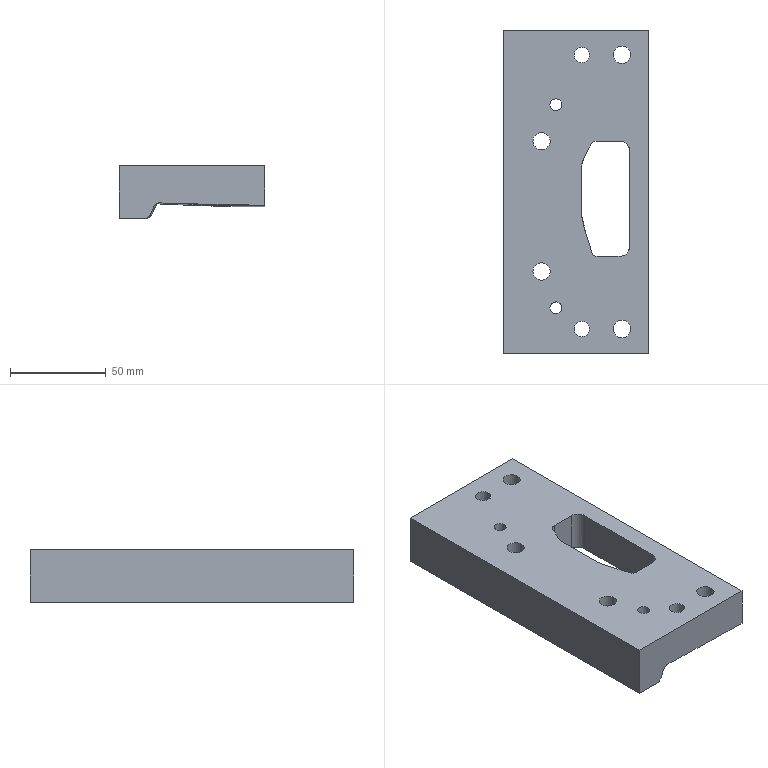Part | STEP file | 431_id654_x_t | 1 solid | 66 faces | volume 227160 mm3 | spline 26 | plane 21 | cylinder 19 | commonest cylinder face diameters 9 x4 10 x4 14 x4 6 x3 6.2 x2 8 x2